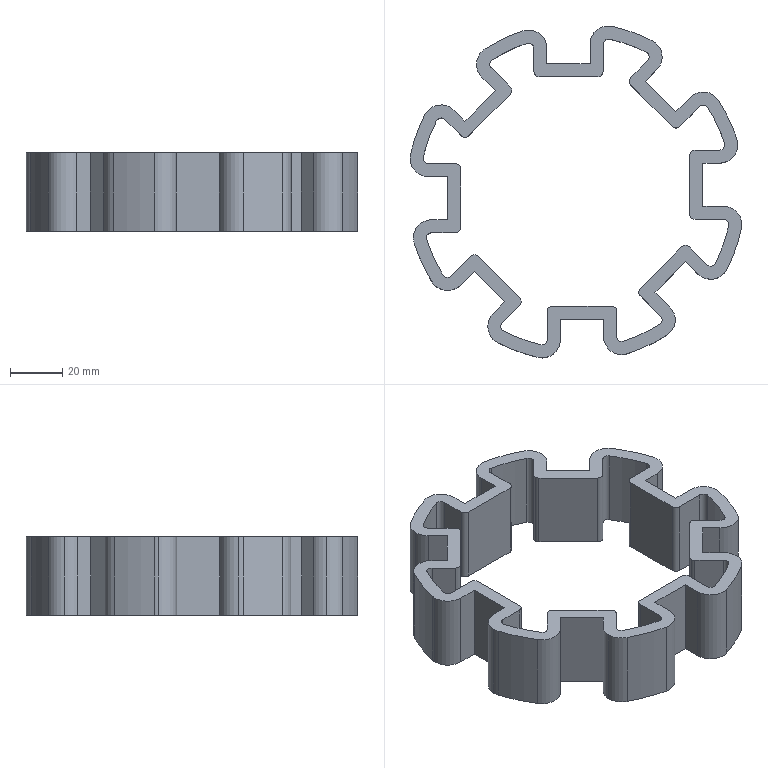Part | SolidWorks | features BaseBody 1 | 1 solid | 127 faces | box 127.193 x 127.193 x 30 mm | volume 86917 mm3 | cylinder 76 | plane 51 | commonest cylinder face diameters 4 x38 14 x20 120 x8 130 x8 1.542 x2